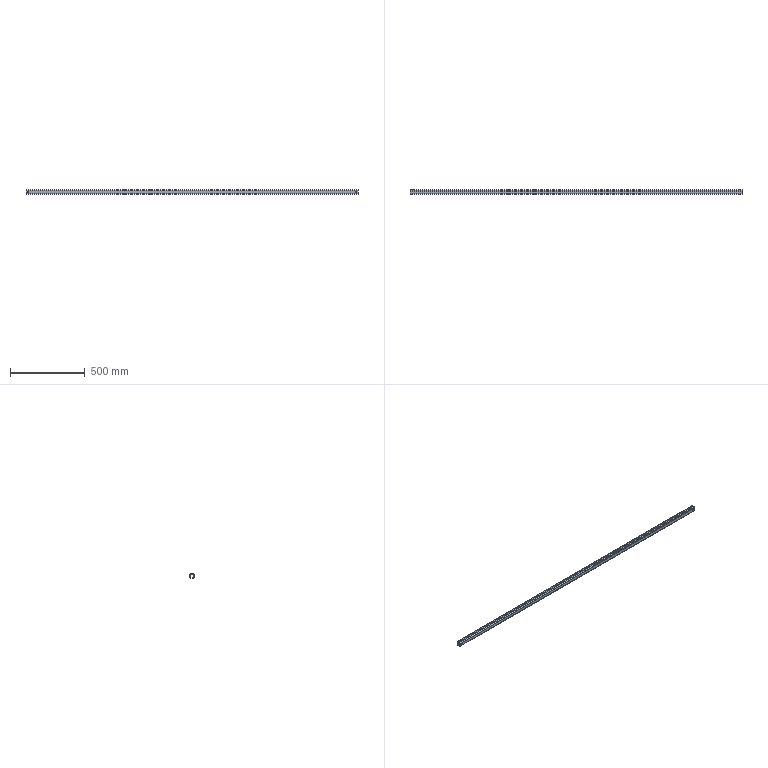Part | NX | features solid 2 | 1 solid | 30 faces | box 2220 x 30 x 30 mm | volume 666162 mm3 | cylinder 16 | plane 14 | commonest cylinder face diameters 6 x4 10 x4 12 x4 15 x4
STEP:
#1=CARTESIAN_POINT('',(1095.,-620.,42.5));
#2=VERTEX_POINT('',#1);
#3=CARTESIAN_POINT('',(1095.,-623.,42.5));
#4=VERTEX_POINT('',#3);
#5=CARTESIAN_POINT('',(1095.,-620.,42.5));
#6=DIRECTION('',(0.,-1.,0.));
#7=VECTOR('',#6,1000.);
#8=LINE('',#5,#7);
#9=EDGE_CURVE('',#2,#4,#8,.T.);
#10=ORIENTED_EDGE('',*,*,#9,.F.);
#11=CARTESIAN_POINT('',(1095.,-620.,57.5));
#12=VERTEX_POINT('',#11);
#13=CARTESIAN_POINT('',(1095.,-620.,50.));
#14=DIRECTION('',(0.,-1.,0.));
#15=DIRECTION('',(0.,0.,1.));
#16=AXIS2_PLACEMENT_3D('',#13,#14,#15);
#17=CIRCLE('',#16,7.5);
#18=EDGE_CURVE('',#12,#2,#17,.T.);
#19=ORIENTED_EDGE('',*,*,#18,.F.);
#20=CARTESIAN_POINT('',(1095.,-623.,57.5));
#21=VERTEX_POINT('',#20);
#22=CARTESIAN_POINT('',(1095.,-620.,57.5));
#23=DIRECTION('',(0.,-1.,0.));
#24=VECTOR('',#23,1000.);
#25=LINE('',#22,#24);
#26=EDGE_CURVE('',#21,#12,#25,.F.);
#27=ORIENTED_EDGE('',*,*,#26,.F.);
#28=CARTESIAN_POINT('',(1095.,-623.,50.));
#29=DIRECTION('',(0.,1.,0.));
#30=DIRECTION('',(0.,0.,1.));
#31=AXIS2_PLACEMENT_3D('',#28,#29,#30);
#32=CIRCLE('',#31,7.5);
#33=EDGE_CURVE('',#4,#21,#32,.T.);
#34=ORIENTED_EDGE('',*,*,#33,.F.);
#35=EDGE_LOOP('',(#10,#19,#27,#34));
#36=FACE_BOUND('',#35,.T.);
#37=CARTESIAN_POINT('',(1095.,-620.,50.));
#38=DIRECTION('',(0.,-1.,0.));
#39=DIRECTION('',(0.,0.,1.));
#40=AXIS2_PLACEMENT_3D('',#37,#38,#39);
#41=CYLINDRICAL_SURFACE('',#40,7.5);
#42=ADVANCED_FACE('',(#36),#41,.F.);
#43=CARTESIAN_POINT('',(1095.,-650.,45.));
#44=VERTEX_POINT('',#43);
#45=CARTESIAN_POINT('',(1095.,-647.,45.));
#46=VERTEX_POINT('',#45);
#47=CARTESIAN_POINT('',(1095.,-2849.405,45.));
#48=DIRECTION('',(0.,1.,0.));
#49=VECTOR('',#48,1000.);
#50=LINE('',#47,#49);
#51=EDGE_CURVE('',#44,#46,#50,.T.);
#52=ORIENTED_EDGE('',*,*,#51,.F.);
#53=CARTESIAN_POINT('',(1095.,-650.,55.));
#54=VERTEX_POINT('',#53);
#55=CARTESIAN_POINT('',(1095.,-650.,50.));
#56=DIRECTION('',(0.,-1.,0.));
#57=DIRECTION('',(0.,0.,-1.));
#58=AXIS2_PLACEMENT_3D('',#55,#56,#57);
#59=CIRCLE('',#58,5.);
#60=EDGE_CURVE('',#44,#54,#59,.T.);
#61=ORIENTED_EDGE('',*,*,#60,.T.);
#62=CARTESIAN_POINT('',(1095.,-647.,55.));
#63=VERTEX_POINT('',#62);
#64=CARTESIAN_POINT('',(1095.,-2849.405,55.));
#65=DIRECTION('',(0.,1.,0.));
#66=VECTOR('',#65,1000.);
#67=LINE('',#64,#66);
#68=EDGE_CURVE('',#63,#54,#67,.F.);
#69=ORIENTED_EDGE('',*,*,#68,.F.);
#70=CARTESIAN_POINT('',(1095.,-647.,50.));
#71=DIRECTION('',(0.,-1.,0.));
#72=DIRECTION('',(0.,0.,-1.));
#73=AXIS2_PLACEMENT_3D('',#70,#71,#72);
#74=CIRCLE('',#73,5.);
#75=EDGE_CURVE('',#46,#63,#74,.T.);
#76=ORIENTED_EDGE('',*,*,#75,.F.);
#77=EDGE_LOOP('',(#52,#61,#69,#76));
#78=FACE_BOUND('',#77,.T.);
#79=CARTESIAN_POINT('',(1095.,-2849.405,50.));
#80=DIRECTION('',(0.,1.,0.));
#81=DIRECTION('',(0.,0.,1.));
#82=AXIS2_PLACEMENT_3D('',#79,#80,#81);
#83=CYLINDRICAL_SURFACE('',#82,5.);
#84=ADVANCED_FACE('',(#78),#83,.F.);
#85=CARTESIAN_POINT('',(-1095.,-620.,42.5));
#86=VERTEX_POINT('',#85);
#87=CARTESIAN_POINT('',(-1095.,-623.,42.5));
#88=VERTEX_POINT('',#87);
#89=CARTESIAN_POINT('',(-1095.,-620.,42.5));
#90=DIRECTION('',(0.,-1.,0.));
#91=VECTOR('',#90,1000.);
#92=LINE('',#89,#91);
#93=EDGE_CURVE('',#86,#88,#92,.T.);
#94=ORIENTED_EDGE('',*,*,#93,.F.);
#95=CARTESIAN_POINT('',(-1095.,-620.,57.5));
#96=VERTEX_POINT('',#95);
#97=CARTESIAN_POINT('',(-1095.,-620.,50.));
#98=DIRECTION('',(0.,-1.,0.));
#99=DIRECTION('',(0.,0.,1.));
#100=AXIS2_PLACEMENT_3D('',#97,#98,#99);
#101=CIRCLE('',#100,7.5);
#102=EDGE_CURVE('',#96,#86,#101,.T.);
#103=ORIENTED_EDGE('',*,*,#102,.F.);
#104=CARTESIAN_POINT('',(-1095.,-623.,57.5));
#105=VERTEX_POINT('',#104);
#106=CARTESIAN_POINT('',(-1095.,-620.,57.5));
#107=DIRECTION('',(0.,-1.,0.));
#108=VECTOR('',#107,1000.);
#109=LINE('',#106,#108);
#110=EDGE_CURVE('',#105,#96,#109,.F.);
#111=ORIENTED_EDGE('',*,*,#110,.F.);
#112=CARTESIAN_POINT('',(-1095.,-623.,50.));
#113=DIRECTION('',(0.,1.,0.));
#114=DIRECTION('',(0.,0.,1.));
#115=AXIS2_PLACEMENT_3D('',#112,#113,#114);
#116=CIRCLE('',#115,7.5);
#117=EDGE_CURVE('',#88,#105,#116,.T.);
#118=ORIENTED_EDGE('',*,*,#117,.F.);
#119=EDGE_LOOP('',(#94,#103,#111,#118));
#120=FACE_BOUND('',#119,.T.);
#121=CARTESIAN_POINT('',(-1095.,-620.,50.));
#122=DIRECTION('',(0.,-1.,0.));
#123=DIRECTION('',(0.,0.,1.));
#124=AXIS2_PLACEMENT_3D('',#121,#122,#123);
#125=CYLINDRICAL_SURFACE('',#124,7.5);
#126=ADVANCED_FACE('',(#120),#125,.F.);
#127=CARTESIAN_POINT('',(-1095.,-647.,45.));
#128=VERTEX_POINT('',#127);
#129=CARTESIAN_POINT('',(-1095.,-650.,45.));
#130=VERTEX_POINT('',#129);
#131=CARTESIAN_POINT('',(-1095.,-2849.405,45.));
#132=DIRECTION('',(0.,1.,0.));
#133=VECTOR('',#132,1000.);
#134=LINE('',#131,#133);
#135=EDGE_CURVE('',#128,#130,#134,.F.);
#136=ORIENTED_EDGE('',*,*,#135,.T.);
#137=CARTESIAN_POINT('',(-1095.,-650.,55.));
#138=VERTEX_POINT('',#137);
#139=CARTESIAN_POINT('',(-1095.,-650.,50.));
#140=DIRECTION('',(0.,-1.,0.));
#141=DIRECTION('',(0.,0.,-1.));
#142=AXIS2_PLACEMENT_3D('',#139,#140,#141);
#143=CIRCLE('',#142,5.);
#144=EDGE_CURVE('',#130,#138,#143,.T.);
#145=ORIENTED_EDGE('',*,*,#144,.T.);
#146=CARTESIAN_POINT('',(-1095.,-647.,55.));
#147=VERTEX_POINT('',#146);
#148=CARTESIAN_POINT('',(-1095.,-2849.405,55.));
#149=DIRECTION('',(0.,1.,0.));
#150=VECTOR('',#149,1000.);
#151=LINE('',#148,#150);
#152=EDGE_CURVE('',#138,#147,#151,.T.);
#153=ORIENTED_EDGE('',*,*,#152,.T.);
#154=CARTESIAN_POINT('',(-1095.,-647.,50.));
#155=DIRECTION('',(0.,-1.,0.));
#156=DIRECTION('',(0.,0.,-1.));
#157=AXIS2_PLACEMENT_3D('',#154,#155,#156);
#158=CIRCLE('',#157,5.);
#159=EDGE_CURVE('',#128,#147,#158,.T.);
#160=ORIENTED_EDGE('',*,*,#159,.F.);
#161=EDGE_LOOP('',(#136,#145,#153,#160));
#162=FACE_BOUND('',#161,.T.);
#163=CARTESIAN_POINT('',(-1095.,-2849.405,50.));
#164=DIRECTION('',(0.,1.,0.));
#165=DIRECTION('',(0.,0.,1.));
#166=AXIS2_PLACEMENT_3D('',#163,#164,#165);
#167=CYLINDRICAL_SURFACE('',#166,5.);
#168=ADVANCED_FACE('',(#162),#167,.F.);
#169=CARTESIAN_POINT('',(1110.,-626.,62.));
#170=VERTEX_POINT('',#169);
#171=CARTESIAN_POINT('',(1110.,-634.99,62.));
#172=VERTEX_POINT('',#171);
#173=CARTESIAN_POINT('',(1110.,-620.,62.));
#174=DIRECTION('',(0.,-1.,0.));
#175=VECTOR('',#174,1000.);
#176=LINE('',#173,#175);
#177=EDGE_CURVE('',#170,#172,#176,.T.);
#178=ORIENTED_EDGE('',*,*,#177,.T.);
#179=CARTESIAN_POINT('',(-1110.,-634.99,62.));
#180=VERTEX_POINT('',#179);
#181=CARTESIAN_POINT('',(-1110.,-634.99,62.));
#182=DIRECTION('',(1.,0.,0.));
#183=VECTOR('',#182,1000.);
#184=LINE('',#181,#183);
#185=EDGE_CURVE('',#180,#172,#184,.T.);
#186=ORIENTED_EDGE('',*,*,#185,.F.);
#187=CARTESIAN_POINT('',(-1110.,-626.,62.));
#188=VERTEX_POINT('',#187);
#189=CARTESIAN_POINT('',(-1110.,-620.,62.));
#190=DIRECTION('',(0.,-1.,0.));
#191=VECTOR('',#190,1000.);
#192=LINE('',#189,#191);
#193=EDGE_CURVE('',#188,#180,#192,.T.);
#194=ORIENTED_EDGE('',*,*,#193,.F.);
#195=CARTESIAN_POINT('',(-1110.,-626.,62.));
#196=DIRECTION('',(1.,0.,0.));
#197=VECTOR('',#196,1000.);
#198=LINE('',#195,#197);
#199=EDGE_CURVE('',#188,#170,#198,.T.);
#200=ORIENTED_EDGE('',*,*,#199,.T.);
#201=EDGE_LOOP('',(#178,#186,#194,#200));
#202=FACE_BOUND('',#201,.T.);
#203=CARTESIAN_POINT('',(-1110.,-620.,62.));
#204=DIRECTION('',(0.,0.,1.));
#205=DIRECTION('',(0.,-1.,0.));
#206=AXIS2_PLACEMENT_3D('',#203,#204,#205);
#207=PLANE('',#206);
#208=ADVANCED_FACE('',(#202),#207,.F.);
#209=CARTESIAN_POINT('',(1110.,-623.,59.));
#210=VERTEX_POINT('',#209);
#211=CARTESIAN_POINT('',(1110.,-626.,59.));
#212=DIRECTION('',(1.,0.,0.));
#213=DIRECTION('',(0.,0.,-1.));
#214=AXIS2_PLACEMENT_3D('',#211,#212,#213);
#215=CIRCLE('',#214,3.);
#216=EDGE_CURVE('',#210,#170,#215,.T.);
#217=ORIENTED_EDGE('',*,*,#216,.T.);
#218=ORIENTED_EDGE('',*,*,#199,.F.);
#219=CARTESIAN_POINT('',(-1110.,-623.,59.));
#220=VERTEX_POINT('',#219);
#221=CARTESIAN_POINT('',(-1110.,-626.,59.));
#222=DIRECTION('',(1.,0.,0.));
#223=DIRECTION('',(0.,0.,-1.));
#224=AXIS2_PLACEMENT_3D('',#221,#222,#223);
#225=CIRCLE('',#224,3.);
#226=EDGE_CURVE('',#220,#188,#225,.T.);
#227=ORIENTED_EDGE('',*,*,#226,.F.);
#228=CARTESIAN_POINT('',(-1110.,-623.,59.));
#229=DIRECTION('',(1.,0.,0.));
#230=VECTOR('',#229,1000.);
#231=LINE('',#228,#230);
#232=EDGE_CURVE('',#220,#210,#231,.T.);
#233=ORIENTED_EDGE('',*,*,#232,.T.);
#234=EDGE_LOOP('',(#217,#218,#227,#233));
#235=FACE_BOUND('',#234,.T.);
#236=CARTESIAN_POINT('',(-1110.,-626.,59.));
#237=DIRECTION('',(1.,0.,0.));
#238=DIRECTION('',(0.,0.,-1.));
#239=AXIS2_PLACEMENT_3D('',#236,#237,#238);
#240=CYLINDRICAL_SURFACE('',#239,3.);
#241=ADVANCED_FACE('',(#235),#240,.F.);
#242=CARTESIAN_POINT('',(-1095.,-623.,50.));
#243=DIRECTION('',(0.,1.,0.));
#244=DIRECTION('',(0.,0.,1.));
#245=AXIS2_PLACEMENT_3D('',#242,#243,#244);
#246=CIRCLE('',#245,7.5);
#247=EDGE_CURVE('',#105,#88,#246,.T.);
#248=ORIENTED_EDGE('',*,*,#247,.T.);
#249=ORIENTED_EDGE('',*,*,#117,.T.);
#250=EDGE_LOOP('',(#248,#249));
#251=FACE_BOUND('',#250,.T.);
#252=CARTESIAN_POINT('',(1095.,-623.,50.));
#253=DIRECTION('',(0.,1.,0.));
#254=DIRECTION('',(0.,0.,1.));
#255=AXIS2_PLACEMENT_3D('',#252,#253,#254);
#256=CIRCLE('',#255,7.5);
#257=EDGE_CURVE('',#21,#4,#256,.T.);
#258=ORIENTED_EDGE('',*,*,#257,.T.);
#259=ORIENTED_EDGE('',*,*,#33,.T.);
#260=EDGE_LOOP('',(#258,#259));
#261=FACE_BOUND('',#260,.T.);
#262=CARTESIAN_POINT('',(1110.,-623.,41.));
#263=VERTEX_POINT('',#262);
#264=CARTESIAN_POINT('',(1110.,-623.,35.));
#265=DIRECTION('',(0.,0.,1.));
#266=VECTOR('',#265,1000.);
#267=LINE('',#264,#266);
#268=EDGE_CURVE('',#263,#210,#267,.T.);
#269=ORIENTED_EDGE('',*,*,#268,.T.);
#270=ORIENTED_EDGE('',*,*,#232,.F.);
#271=CARTESIAN_POINT('',(-1110.,-623.,41.));
#272=VERTEX_POINT('',#271);
#273=CARTESIAN_POINT('',(-1110.,-623.,35.));
#274=DIRECTION('',(0.,0.,1.));
#275=VECTOR('',#274,1000.);
#276=LINE('',#273,#275);
#277=EDGE_CURVE('',#272,#220,#276,.T.);
#278=ORIENTED_EDGE('',*,*,#277,.F.);
#279=CARTESIAN_POINT('',(-1110.,-623.,41.));
#280=DIRECTION('',(1.,0.,0.));
#281=VECTOR('',#280,1000.);
#282=LINE('',#279,#281);
#283=EDGE_CURVE('',#272,#263,#282,.T.);
#284=ORIENTED_EDGE('',*,*,#283,.T.);
#285=EDGE_LOOP('',(#269,#270,#278,#284));
#286=FACE_BOUND('',#285,.T.);
#287=CARTESIAN_POINT('',(-1110.,-623.,35.));
#288=DIRECTION('',(0.,1.,0.));
#289=DIRECTION('',(0.,0.,-1.));
#290=AXIS2_PLACEMENT_3D('',#287,#288,#289);
#291=PLANE('',#290);
#292=ADVANCED_FACE('',(#251,#261,#286),#291,.F.);
#293=CARTESIAN_POINT('',(1110.,-626.,38.));
#294=VERTEX_POINT('',#293);
#295=CARTESIAN_POINT('',(1110.,-626.,41.));
#296=DIRECTION('',(1.,0.,0.));
#297=DIRECTION('',(0.,0.,-1.));
#298=AXIS2_PLACEMENT_3D('',#295,#296,#297);
#299=CIRCLE('',#298,3.);
#300=EDGE_CURVE('',#294,#263,#299,.T.);
#301=ORIENTED_EDGE('',*,*,#300,.T.);
#302=ORIENTED_EDGE('',*,*,#283,.F.);
#303=CARTESIAN_POINT('',(-1110.,-626.,38.));
#304=VERTEX_POINT('',#303);
#305=CARTESIAN_POINT('',(-1110.,-626.,41.));
#306=DIRECTION('',(1.,0.,0.));
#307=DIRECTION('',(0.,0.,-1.));
#308=AXIS2_PLACEMENT_3D('',#305,#306,#307);
#309=CIRCLE('',#308,3.);
#310=EDGE_CURVE('',#304,#272,#309,.T.);
#311=ORIENTED_EDGE('',*,*,#310,.F.);
#312=CARTESIAN_POINT('',(-1110.,-626.,38.));
#313=DIRECTION('',(1.,0.,0.));
#314=VECTOR('',#313,1000.);
#315=LINE('',#312,#314);
#316=EDGE_CURVE('',#304,#294,#315,.T.);
#317=ORIENTED_EDGE('',*,*,#316,.T.);
#318=EDGE_LOOP('',(#301,#302,#311,#317));
#319=FACE_BOUND('',#318,.T.);
#320=CARTESIAN_POINT('',(-1110.,-626.,41.));
#321=DIRECTION('',(1.,0.,0.));
#322=DIRECTION('',(0.,0.,-1.));
#323=AXIS2_PLACEMENT_3D('',#320,#321,#322);
#324=CYLINDRICAL_SURFACE('',#323,3.);
#325=ADVANCED_FACE('',(#319),#324,.F.);
#326=CARTESIAN_POINT('',(1110.,-644.,38.));
#327=VERTEX_POINT('',#326);
#328=CARTESIAN_POINT('',(1110.,-650.,38.));
#329=DIRECTION('',(0.,1.,0.));
#330=VECTOR('',#329,1000.);
#331=LINE('',#328,#330);
#332=EDGE_CURVE('',#327,#294,#331,.T.);
#333=ORIENTED_EDGE('',*,*,#332,.T.);
#334=ORIENTED_EDGE('',*,*,#316,.F.);
#335=CARTESIAN_POINT('',(-1110.,-644.,38.));
#336=VERTEX_POINT('',#335);
#337=CARTESIAN_POINT('',(-1110.,-650.,38.));
#338=DIRECTION('',(0.,1.,0.));
#339=VECTOR('',#338,1000.);
#340=LINE('',#337,#339);
#341=EDGE_CURVE('',#336,#304,#340,.T.);
#342=ORIENTED_EDGE('',*,*,#341,.F.);
#343=CARTESIAN_POINT('',(-1110.,-644.,38.));
#344=DIRECTION('',(1.,0.,0.));
#345=VECTOR('',#344,1000.);
#346=LINE('',#343,#345);
#347=EDGE_CURVE('',#336,#327,#346,.T.);
#348=ORIENTED_EDGE('',*,*,#347,.T.);
#349=EDGE_LOOP('',(#333,#334,#342,#348));
#350=FACE_BOUND('',#349,.T.);
#351=CARTESIAN_POINT('',(-1110.,-650.,38.));
#352=DIRECTION('',(0.,0.,-1.));
#353=DIRECTION('',(0.,-1.,0.));
#354=AXIS2_PLACEMENT_3D('',#351,#352,#353);
#355=PLANE('',#354);
#356=ADVANCED_FACE('',(#350),#355,.F.);
#357=CARTESIAN_POINT('',(1110.,-647.,41.));
#358=VERTEX_POINT('',#357);
#359=CARTESIAN_POINT('',(1110.,-644.,41.));
#360=DIRECTION('',(1.,0.,0.));
#361=DIRECTION('',(0.,0.,-1.));
#362=AXIS2_PLACEMENT_3D('',#359,#360,#361);
#363=CIRCLE('',#362,3.);
#364=EDGE_CURVE('',#358,#327,#363,.T.);
#365=ORIENTED_EDGE('',*,*,#364,.T.);
#366=ORIENTED_EDGE('',*,*,#347,.F.);
#367=CARTESIAN_POINT('',(-1110.,-647.,41.));
#368=VERTEX_POINT('',#367);
#369=CARTESIAN_POINT('',(-1110.,-644.,41.));
#370=DIRECTION('',(1.,0.,0.));
#371=DIRECTION('',(0.,0.,-1.));
#372=AXIS2_PLACEMENT_3D('',#369,#370,#371);
#373=CIRCLE('',#372,3.);
#374=EDGE_CURVE('',#368,#336,#373,.T.);
#375=ORIENTED_EDGE('',*,*,#374,.F.);
#376=CARTESIAN_POINT('',(-1110.,-647.,41.));
#377=DIRECTION('',(1.,0.,0.));
#378=VECTOR('',#377,1000.);
#379=LINE('',#376,#378);
#380=EDGE_CURVE('',#368,#358,#379,.T.);
#381=ORIENTED_EDGE('',*,*,#380,.T.);
#382=EDGE_LOOP('',(#365,#366,#375,#381));
#383=FACE_BOUND('',#382,.T.);
#384=CARTESIAN_POINT('',(-1110.,-644.,41.));
#385=DIRECTION('',(1.,0.,0.));
#386=DIRECTION('',(0.,0.,-1.));
#387=AXIS2_PLACEMENT_3D('',#384,#385,#386);
#388=CYLINDRICAL_SURFACE('',#387,3.);
#389=ADVANCED_FACE('',(#383),#388,.F.);
#390=CARTESIAN_POINT('',(-1095.,-647.,50.));
#391=DIRECTION('',(0.,-1.,0.));
#392=DIRECTION('',(0.,0.,-1.));
#393=AXIS2_PLACEMENT_3D('',#390,#391,#392);
#394=CIRCLE('',#393,5.);
#395=EDGE_CURVE('',#147,#128,#394,.T.);
#396=ORIENTED_EDGE('',*,*,#395,.T.);
#397=ORIENTED_EDGE('',*,*,#159,.T.);
#398=EDGE_LOOP('',(#396,#397));
#399=FACE_BOUND('',#398,.T.);
#400=CARTESIAN_POINT('',(1095.,-647.,50.));
#401=DIRECTION('',(0.,-1.,0.));
#402=DIRECTION('',(0.,0.,-1.));
#403=AXIS2_PLACEMENT_3D('',#400,#401,#402);
#404=CIRCLE('',#403,5.);
#405=EDGE_CURVE('',#63,#46,#404,.T.);
#406=ORIENTED_EDGE('',*,*,#405,.T.);
#407=ORIENTED_EDGE('',*,*,#75,.T.);
#408=EDGE_LOOP('',(#406,#407));
#409=FACE_BOUND('',#408,.T.);
#410=CARTESIAN_POINT('',(1110.,-647.,59.));
#411=VERTEX_POINT('',#410);
#412=CARTESIAN_POINT('',(1110.,-647.,65.));
#413=DIRECTION('',(0.,0.,-1.));
#414=VECTOR('',#413,1000.);
#415=LINE('',#412,#414);
#416=EDGE_CURVE('',#411,#358,#415,.T.);
#417=ORIENTED_EDGE('',*,*,#416,.T.);
#418=ORIENTED_EDGE('',*,*,#380,.F.);
#419=CARTESIAN_POINT('',(-1110.,-647.,59.));
#420=VERTEX_POINT('',#419);
#421=CARTESIAN_POINT('',(-1110.,-647.,65.));
#422=DIRECTION('',(0.,0.,-1.));
#423=VECTOR('',#422,1000.);
#424=LINE('',#421,#423);
#425=EDGE_CURVE('',#420,#368,#424,.T.);
#426=ORIENTED_EDGE('',*,*,#425,.F.);
#427=CARTESIAN_POINT('',(-1110.,-647.,59.));
#428=DIRECTION('',(1.,0.,0.));
#429=VECTOR('',#428,1000.);
#430=LINE('',#427,#429);
#431=EDGE_CURVE('',#420,#411,#430,.T.);
#432=ORIENTED_EDGE('',*,*,#431,.T.);
#433=EDGE_LOOP('',(#417,#418,#426,#432));
#434=FACE_BOUND('',#433,.T.);
#435=CARTESIAN_POINT('',(-1110.,-647.,65.));
#436=DIRECTION('',(0.,-1.,0.));
#437=DIRECTION('',(0.,0.,-1.));
#438=AXIS2_PLACEMENT_3D('',#435,#436,#437);
#439=PLANE('',#438);
#440=ADVANCED_FACE('',(#399,#409,#434),#439,.F.);
#441=CARTESIAN_POINT('',(1110.,-644.,62.));
#442=VERTEX_POINT('',#441);
#443=CARTESIAN_POINT('',(1110.,-644.,59.));
#444=DIRECTION('',(1.,0.,0.));
#445=DIRECTION('',(0.,0.,-1.));
#446=AXIS2_PLACEMENT_3D('',#443,#444,#445);
#447=CIRCLE('',#446,3.);
#448=EDGE_CURVE('',#442,#411,#447,.T.);
#449=ORIENTED_EDGE('',*,*,#448,.T.);
#450=ORIENTED_EDGE('',*,*,#431,.F.);
#451=CARTESIAN_POINT('',(-1110.,-644.,62.));
#452=VERTEX_POINT('',#451);
#453=CARTESIAN_POINT('',(-1110.,-644.,59.));
#454=DIRECTION('',(1.,0.,0.));
#455=DIRECTION('',(0.,0.,-1.));
#456=AXIS2_PLACEMENT_3D('',#453,#454,#455);
#457=CIRCLE('',#456,3.);
#458=EDGE_CURVE('',#452,#420,#457,.T.);
#459=ORIENTED_EDGE('',*,*,#458,.F.);
#460=CARTESIAN_POINT('',(-1110.,-644.,62.));
#461=DIRECTION('',(1.,0.,0.));
#462=VECTOR('',#461,1000.);
#463=LINE('',#460,#462);
#464=EDGE_CURVE('',#452,#442,#463,.T.);
#465=ORIENTED_EDGE('',*,*,#464,.T.);
#466=EDGE_LOOP('',(#449,#450,#459,#465));
#467=FACE_BOUND('',#466,.T.);
#468=CARTESIAN_POINT('',(-1110.,-644.,59.));
#469=DIRECTION('',(1.,0.,0.));
#470=DIRECTION('',(0.,0.,-1.));
#471=AXIS2_PLACEMENT_3D('',#468,#469,#470);
#472=CYLINDRICAL_SURFACE('',#471,3.);
#473=ADVANCED_FACE('',(#467),#472,.F.);
#474=CARTESIAN_POINT('',(1110.,-635.01,62.));
#475=VERTEX_POINT('',#474);
#476=CARTESIAN_POINT('',(1110.,-635.01,62.));
#477=DIRECTION('',(0.,-1.,0.));
#478=VECTOR('',#477,1000.);
#479=LINE('',#476,#478);
#480=EDGE_CURVE('',#475,#442,#479,.T.);
#481=ORIENTED_EDGE('',*,*,#480,.T.);
#482=ORIENTED_EDGE('',*,*,#464,.F.);
#483=CARTESIAN_POINT('',(-1110.,-635.01,62.));
#484=VERTEX_POINT('',#483);
#485=CARTESIAN_POINT('',(-1110.,-635.01,62.));
#486=DIRECTION('',(0.,-1.,0.));
#487=VECTOR('',#486,1000.);
#488=LINE('',#485,#487);
#489=EDGE_CURVE('',#484,#452,#488,.T.);
#490=ORIENTED_EDGE('',*,*,#489,.F.);
#491=CARTESIAN_POINT('',(-1110.,-635.01,62.));
#492=DIRECTION('',(1.,0.,0.));
#493=VECTOR('',#492,1000.);
#494=LINE('',#491,#493);
#495=EDGE_CURVE('',#484,#475,#494,.T.);
#496=ORIENTED_EDGE('',*,*,#495,.T.);
#497=EDGE_LOOP('',(#481,#482,#490,#496));
#498=FACE_BOUND('',#497,.T.);
#499=CARTESIAN_POINT('',(-1110.,-635.01,62.));
#500=DIRECTION('',(0.,0.,1.));
#501=DIRECTION('',(0.,-1.,0.));
#502=AXIS2_PLACEMENT_3D('',#499,#500,#501);
#503=PLANE('',#502);
#504=ADVANCED_FACE('',(#498),#503,.F.);
#505=CARTESIAN_POINT('',(1110.,-626.,65.));
#506=VERTEX_POINT('',#505);
#507=CARTESIAN_POINT('',(1110.,-634.99,65.));
#508=VERTEX_POINT('',#507);
#509=CARTESIAN_POINT('',(1110.,-620.,65.));
#510=DIRECTION('',(0.,-1.,0.));
#511=VECTOR('',#510,1000.);
#512=LINE('',#509,#511);
#513=EDGE_CURVE('',#506,#508,#512,.T.);
#514=ORIENTED_EDGE('',*,*,#513,.F.);
#515=CARTESIAN_POINT('',(-1110.,-626.,65.));
#516=VERTEX_POINT('',#515);
#517=CARTESIAN_POINT('',(-1110.,-626.,65.));
#518=DIRECTION('',(1.,0.,0.));
#519=VECTOR('',#518,1000.);
#520=LINE('',#517,#519);
#521=EDGE_CURVE('',#516,#506,#520,.T.);
#522=ORIENTED_EDGE('',*,*,#521,.F.);
#523=CARTESIAN_POINT('',(-1110.,-634.99,65.));
#524=VERTEX_POINT('',#523);
#525=CARTESIAN_POINT('',(-1110.,-620.,65.));
#526=DIRECTION('',(0.,-1.,0.));
#527=VECTOR('',#526,1000.);
#528=LINE('',#525,#527);
#529=EDGE_CURVE('',#516,#524,#528,.T.);
#530=ORIENTED_EDGE('',*,*,#529,.T.);
#531=CARTESIAN_POINT('',(-1110.,-634.99,65.));
#532=DIRECTION('',(1.,0.,0.));
#533=VECTOR('',#532,1000.);
#534=LINE('',#531,#533);
#535=EDGE_CURVE('',#524,#508,#534,.T.);
#536=ORIENTED_EDGE('',*,*,#535,.T.);
#537=EDGE_LOOP('',(#514,#522,#530,#536));
#538=FACE_BOUND('',#537,.T.);
#539=CARTESIAN_POINT('',(-1110.,-620.,65.));
#540=DIRECTION('',(0.,0.,1.));
#541=DIRECTION('',(0.,-1.,0.));
#542=AXIS2_PLACEMENT_3D('',#539,#540,#541);
#543=PLANE('',#542);
#544=ADVANCED_FACE('',(#538),#543,.T.);
#545=CARTESIAN_POINT('',(1110.,-620.,59.));
#546=VERTEX_POINT('',#545);
#547=CARTESIAN_POINT('',(1110.,-626.,59.));
#548=DIRECTION('',(1.,0.,0.));
#549=DIRECTION('',(0.,-1.,0.));
#550=AXIS2_PLACEMENT_3D('',#547,#548,#549);
#551=CIRCLE('',#550,6.);
#552=EDGE_CURVE('',#546,#506,#551,.T.);
#553=ORIENTED_EDGE('',*,*,#552,.F.);
#554=CARTESIAN_POINT('',(-1110.,-620.,59.));
#555=VERTEX_POINT('',#554);
#556=CARTESIAN_POINT('',(-1110.,-620.,59.));
#557=DIRECTION('',(1.,0.,0.));
#558=VECTOR('',#557,1000.);
#559=LINE('',#556,#558);
#560=EDGE_CURVE('',#555,#546,#559,.T.);
#561=ORIENTED_EDGE('',*,*,#560,.F.);
#562=CARTESIAN_POINT('',(-1110.,-626.,59.));
#563=DIRECTION('',(1.,0.,0.));
#564=DIRECTION('',(0.,-1.,0.));
#565=AXIS2_PLACEMENT_3D('',#562,#563,#564);
#566=CIRCLE('',#565,6.);
#567=EDGE_CURVE('',#555,#516,#566,.T.);
#568=ORIENTED_EDGE('',*,*,#567,.T.);
#569=ORIENTED_EDGE('',*,*,#521,.T.);
#570=EDGE_LOOP('',(#553,#561,#568,#569));
#571=FACE_BOUND('',#570,.T.);
#572=CARTESIAN_POINT('',(-1110.,-626.,59.));
#573=DIRECTION('',(1.,0.,0.));
#574=DIRECTION('',(0.,0.,-1.));
#575=AXIS2_PLACEMENT_3D('',#572,#573,#574);
#576=CYLINDRICAL_SURFACE('',#575,6.);
#577=ADVANCED_FACE('',(#571),#576,.T.);
#578=ORIENTED_EDGE('',*,*,#102,.T.);
#579=CARTESIAN_POINT('',(-1095.,-620.,50.));
#580=DIRECTION('',(0.,-1.,0.));
#581=DIRECTION('',(0.,0.,1.));
#582=AXIS2_PLACEMENT_3D('',#579,#580,#581);
#583=CIRCLE('',#582,7.5);
#584=EDGE_CURVE('',#86,#96,#583,.T.);
#585=ORIENTED_EDGE('',*,*,#584,.T.);
#586=EDGE_LOOP('',(#578,#585));
#587=FACE_BOUND('',#586,.T.);
#588=ORIENTED_EDGE('',*,*,#18,.T.);
#589=CARTESIAN_POINT('',(1095.,-620.,50.));
#590=DIRECTION('',(0.,-1.,0.));
#591=DIRECTION('',(0.,0.,1.));
#592=AXIS2_PLACEMENT_3D('',#589,#590,#591);
#593=CIRCLE('',#592,7.5);
#594=EDGE_CURVE('',#2,#12,#593,.T.);
#595=ORIENTED_EDGE('',*,*,#594,.T.);
#596=EDGE_LOOP('',(#588,#595));
#597=FACE_BOUND('',#596,.T.);
#598=CARTESIAN_POINT('',(1110.,-620.,41.));
#599=VERTEX_POINT('',#598);
#600=CARTESIAN_POINT('',(1110.,-620.,35.));
#601=DIRECTION('',(0.,0.,1.));
#602=VECTOR('',#601,1000.);
#603=LINE('',#600,#602);
#604=EDGE_CURVE('',#599,#546,#603,.T.);
#605=ORIENTED_EDGE('',*,*,#604,.F.);
#606=CARTESIAN_POINT('',(-1110.,-620.,41.));
#607=VERTEX_POINT('',#606);
#608=CARTESIAN_POINT('',(-1110.,-620.,41.));
#609=DIRECTION('',(1.,0.,0.));
#610=VECTOR('',#609,1000.);
#611=LINE('',#608,#610);
#612=EDGE_CURVE('',#607,#599,#611,.T.);
#613=ORIENTED_EDGE('',*,*,#612,.F.);
#614=CARTESIAN_POINT('',(-1110.,-620.,35.));
#615=DIRECTION('',(0.,0.,1.));
#616=VECTOR('',#615,1000.);
#617=LINE('',#614,#616);
#618=EDGE_CURVE('',#607,#555,#617,.T.);
#619=ORIENTED_EDGE('',*,*,#618,.T.);
#620=ORIENTED_EDGE('',*,*,#560,.T.);
#621=EDGE_LOOP('',(#605,#613,#619,#620));
#622=FACE_BOUND('',#621,.T.);
#623=CARTESIAN_POINT('',(-1110.,-620.,35.));
#624=DIRECTION('',(0.,1.,0.));
#625=DIRECTION('',(0.,0.,-1.));
#626=AXIS2_PLACEMENT_3D('',#623,#624,#625);
#627=PLANE('',#626);
#628=ADVANCED_FACE('',(#587,#597,#622),#627,.T.);
#629=CARTESIAN_POINT('',(1110.,-626.,35.));
#630=VERTEX_POINT('',#629);
#631=CARTESIAN_POINT('',(1110.,-626.,41.));
#632=DIRECTION('',(1.,0.,0.));
#633=DIRECTION('',(0.,-1.,0.));
#634=AXIS2_PLACEMENT_3D('',#631,#632,#633);
#635=CIRCLE('',#634,6.);
#636=EDGE_CURVE('',#630,#599,#635,.T.);
#637=ORIENTED_EDGE('',*,*,#636,.F.);
#638=CARTESIAN_POINT('',(-1110.,-626.,35.));
#639=VERTEX_POINT('',#638);
#640=CARTESIAN_POINT('',(-1110.,-626.,35.));
#641=DIRECTION('',(1.,0.,0.));
#642=VECTOR('',#641,1000.);
#643=LINE('',#640,#642);
#644=EDGE_CURVE('',#639,#630,#643,.T.);
#645=ORIENTED_EDGE('',*,*,#644,.F.);
#646=CARTESIAN_POINT('',(-1110.,-626.,41.));
#647=DIRECTION('',(1.,0.,0.));
#648=DIRECTION('',(0.,-1.,0.));
#649=AXIS2_PLACEMENT_3D('',#646,#647,#648);
#650=CIRCLE('',#649,6.);
#651=EDGE_CURVE('',#639,#607,#650,.T.);
#652=ORIENTED_EDGE('',*,*,#651,.T.);
#653=ORIENTED_EDGE('',*,*,#612,.T.);
#654=EDGE_LOOP('',(#637,#645,#652,#653));
#655=FACE_BOUND('',#654,.T.);
#656=CARTESIAN_POINT('',(-1110.,-626.,41.));
#657=DIRECTION('',(1.,0.,0.));
#658=DIRECTION('',(0.,0.,-1.));
#659=AXIS2_PLACEMENT_3D('',#656,#657,#658);
#660=CYLINDRICAL_SURFACE('',#659,6.);
#661=ADVANCED_FACE('',(#655),#660,.T.);
#662=CARTESIAN_POINT('',(1110.,-644.,35.));
#663=VERTEX_POINT('',#662);
#664=CARTESIAN_POINT('',(1110.,-650.,35.));
#665=DIRECTION('',(0.,1.,0.));
#666=VECTOR('',#665,1000.);
#667=LINE('',#664,#666);
#668=EDGE_CURVE('',#663,#630,#667,.T.);
#669=ORIENTED_EDGE('',*,*,#668,.F.);
#670=CARTESIAN_POINT('',(-1110.,-644.,35.));
#671=VERTEX_POINT('',#670);
#672=CARTESIAN_POINT('',(-1110.,-644.,35.));
#673=DIRECTION('',(1.,0.,0.));
#674=VECTOR('',#673,1000.);
#675=LINE('',#672,#674);
#676=EDGE_CURVE('',#671,#663,#675,.T.);
#677=ORIENTED_EDGE('',*,*,#676,.F.);
#678=CARTESIAN_POINT('',(-1110.,-650.,35.));
#679=DIRECTION('',(0.,1.,0.));
#680=VECTOR('',#679,1000.);
#681=LINE('',#678,#680);
#682=EDGE_CURVE('',#671,#639,#681,.T.);
#683=ORIENTED_EDGE('',*,*,#682,.T.);
#684=ORIENTED_EDGE('',*,*,#644,.T.);
#685=EDGE_LOOP('',(#669,#677,#683,#684));
#686=FACE_BOUND('',#685,.T.);
#687=CARTESIAN_POINT('',(-1110.,-650.,35.));
#688=DIRECTION('',(0.,0.,-1.));
#689=DIRECTION('',(0.,-1.,0.));
#690=AXIS2_PLACEMENT_3D('',#687,#688,#689);
#691=PLANE('',#690);
#692=ADVANCED_FACE('',(#686),#691,.T.);
#693=CARTESIAN_POINT('',(1110.,-650.,41.));
#694=VERTEX_POINT('',#693);
#695=CARTESIAN_POINT('',(1110.,-644.,41.));
#696=DIRECTION('',(1.,0.,0.));
#697=DIRECTION('',(0.,-1.,0.));
#698=AXIS2_PLACEMENT_3D('',#695,#696,#697);
#699=CIRCLE('',#698,6.);
#700=EDGE_CURVE('',#694,#663,#699,.T.);
#701=ORIENTED_EDGE('',*,*,#700,.F.);
#702=CARTESIAN_POINT('',(-1110.,-650.,41.));
#703=VERTEX_POINT('',#702);
#704=CARTESIAN_POINT('',(-1110.,-650.,41.));
#705=DIRECTION('',(1.,0.,0.));
#706=VECTOR('',#705,1000.);
#707=LINE('',#704,#706);
#708=EDGE_CURVE('',#703,#694,#707,.T.);
#709=ORIENTED_EDGE('',*,*,#708,.F.);
#710=CARTESIAN_POINT('',(-1110.,-644.,41.));
#711=DIRECTION('',(1.,0.,0.));
#712=DIRECTION('',(0.,-1.,0.));
#713=AXIS2_PLACEMENT_3D('',#710,#711,#712);
#714=CIRCLE('',#713,6.);
#715=EDGE_CURVE('',#703,#671,#714,.T.);
#716=ORIENTED_EDGE('',*,*,#715,.T.);
#717=ORIENTED_EDGE('',*,*,#676,.T.);
#718=EDGE_LOOP('',(#701,#709,#716,#717));
#719=FACE_BOUND('',#718,.T.);
#720=CARTESIAN_POINT('',(-1110.,-644.,41.));
#721=DIRECTION('',(1.,0.,0.));
#722=DIRECTION('',(0.,0.,-1.));
#723=AXIS2_PLACEMENT_3D('',#720,#721,#722);
#724=CYLINDRICAL_SURFACE('',#723,6.);
#725=ADVANCED_FACE('',(#719),#724,.T.);
#726=CARTESIAN_POINT('',(-1095.,-650.,50.));
#727=DIRECTION('',(0.,-1.,0.));
#728=DIRECTION('',(0.,0.,-1.));
#729=AXIS2_PLACEMENT_3D('',#726,#727,#728);
#730=CIRCLE('',#729,5.);
#731=EDGE_CURVE('',#138,#130,#730,.T.);
#732=ORIENTED_EDGE('',*,*,#731,.F.);
#733=ORIENTED_EDGE('',*,*,#144,.F.);
#734=EDGE_LOOP('',(#732,#733));
#735=FACE_BOUND('',#734,.T.);
#736=CARTESIAN_POINT('',(1095.,-650.,50.));
#737=DIRECTION('',(0.,-1.,0.));
#738=DIRECTION('',(0.,0.,-1.));
#739=AXIS2_PLACEMENT_3D('',#736,#737,#738);
#740=CIRCLE('',#739,5.);
#741=EDGE_CURVE('',#54,#44,#740,.T.);
#742=ORIENTED_EDGE('',*,*,#741,.F.);
#743=ORIENTED_EDGE('',*,*,#60,.F.);
#744=EDGE_LOOP('',(#742,#743));
#745=FACE_BOUND('',#744,.T.);
#746=CARTESIAN_POINT('',(1110.,-650.,59.));
#747=VERTEX_POINT('',#746);
#748=CARTESIAN_POINT('',(1110.,-650.,65.));
#749=DIRECTION('',(0.,0.,-1.));
#750=VECTOR('',#749,1000.);
#751=LINE('',#748,#750);
#752=EDGE_CURVE('',#747,#694,#751,.T.);
#753=ORIENTED_EDGE('',*,*,#752,.F.);
#754=CARTESIAN_POINT('',(-1110.,-650.,59.));
#755=VERTEX_POINT('',#754);
#756=CARTESIAN_POINT('',(-1110.,-650.,59.));
#757=DIRECTION('',(1.,0.,0.));
#758=VECTOR('',#757,1000.);
#759=LINE('',#756,#758);
#760=EDGE_CURVE('',#755,#747,#759,.T.);
#761=ORIENTED_EDGE('',*,*,#760,.F.);
#762=CARTESIAN_POINT('',(-1110.,-650.,65.));
#763=DIRECTION('',(0.,0.,-1.));
#764=VECTOR('',#763,1000.);
#765=LINE('',#762,#764);
#766=EDGE_CURVE('',#755,#703,#765,.T.);
#767=ORIENTED_EDGE('',*,*,#766,.T.);
#768=ORIENTED_EDGE('',*,*,#708,.T.);
#769=EDGE_LOOP('',(#753,#761,#767,#768));
#770=FACE_BOUND('',#769,.T.);
#771=CARTESIAN_POINT('',(-1110.,-650.,65.));
#772=DIRECTION('',(0.,-1.,0.));
#773=DIRECTION('',(0.,0.,-1.));
#774=AXIS2_PLACEMENT_3D('',#771,#772,#773);
#775=PLANE('',#774);
#776=ADVANCED_FACE('',(#735,#745,#770),#775,.T.);
#777=CARTESIAN_POINT('',(1110.,-644.,65.));
#778=VERTEX_POINT('',#777);
#779=CARTESIAN_POINT('',(1110.,-644.,59.));
#780=DIRECTION('',(1.,0.,0.));
#781=DIRECTION('',(0.,-1.,0.));
#782=AXIS2_PLACEMENT_3D('',#779,#780,#781);
#783=CIRCLE('',#782,6.);
#784=EDGE_CURVE('',#778,#747,#783,.T.);
#785=ORIENTED_EDGE('',*,*,#784,.F.);
#786=CARTESIAN_POINT('',(-1110.,-644.,65.));
#787=VERTEX_POINT('',#786);
#788=CARTESIAN_POINT('',(-1110.,-644.,65.));
#789=DIRECTION('',(1.,0.,0.));
#790=VECTOR('',#789,1000.);
#791=LINE('',#788,#790);
#792=EDGE_CURVE('',#787,#778,#791,.T.);
#793=ORIENTED_EDGE('',*,*,#792,.F.);
#794=CARTESIAN_POINT('',(-1110.,-644.,59.));
#795=DIRECTION('',(1.,0.,0.));
#796=DIRECTION('',(0.,-1.,0.));
#797=AXIS2_PLACEMENT_3D('',#794,#795,#796);
#798=CIRCLE('',#797,6.);
#799=EDGE_CURVE('',#787,#755,#798,.T.);
#800=ORIENTED_EDGE('',*,*,#799,.T.);
#801=ORIENTED_EDGE('',*,*,#760,.T.);
#802=EDGE_LOOP('',(#785,#793,#800,#801));
#803=FACE_BOUND('',#802,.T.);
#804=CARTESIAN_POINT('',(-1110.,-644.,59.));
#805=DIRECTION('',(1.,0.,0.));
#806=DIRECTION('',(0.,0.,-1.));
#807=AXIS2_PLACEMENT_3D('',#804,#805,#806);
#808=CYLINDRICAL_SURFACE('',#807,6.);
#809=ADVANCED_FACE('',(#803),#808,.T.);
#810=CARTESIAN_POINT('',(1110.,-635.01,65.));
#811=VERTEX_POINT('',#810);
#812=CARTESIAN_POINT('',(1110.,-635.01,65.));
#813=DIRECTION('',(0.,-1.,0.));
#814=VECTOR('',#813,1000.);
#815=LINE('',#812,#814);
#816=EDGE_CURVE('',#811,#778,#815,.T.);
#817=ORIENTED_EDGE('',*,*,#816,.F.);
#818=CARTESIAN_POINT('',(-1110.,-635.01,65.));
#819=VERTEX_POINT('',#818);
#820=CARTESIAN_POINT('',(-1110.,-635.01,65.));
#821=DIRECTION('',(1.,0.,0.));
#822=VECTOR('',#821,1000.);
#823=LINE('',#820,#822);
#824=EDGE_CURVE('',#819,#811,#823,.T.);
#825=ORIENTED_EDGE('',*,*,#824,.F.);
#826=CARTESIAN_POINT('',(-1110.,-635.01,65.));
#827=DIRECTION('',(0.,-1.,0.));
#828=VECTOR('',#827,1000.);
#829=LINE('',#826,#828);
#830=EDGE_CURVE('',#819,#787,#829,.T.);
#831=ORIENTED_EDGE('',*,*,#830,.T.);
#832=ORIENTED_EDGE('',*,*,#792,.T.);
#833=EDGE_LOOP('',(#817,#825,#831,#832));
#834=FACE_BOUND('',#833,.T.);
#835=CARTESIAN_POINT('',(-1110.,-635.01,65.));
#836=DIRECTION('',(0.,0.,1.));
#837=DIRECTION('',(0.,-1.,0.));
#838=AXIS2_PLACEMENT_3D('',#835,#836,#837);
#839=PLANE('',#838);
#840=ADVANCED_FACE('',(#834),#839,.T.);
#841=ORIENTED_EDGE('',*,*,#495,.F.);
#842=CARTESIAN_POINT('',(-1110.,-635.01,65.));
#843=DIRECTION('',(0.,0.,1.));
#844=VECTOR('',#843,1000.);
#845=LINE('',#842,#844);
#846=EDGE_CURVE('',#484,#819,#845,.T.);
#847=ORIENTED_EDGE('',*,*,#846,.T.);
#848=ORIENTED_EDGE('',*,*,#824,.T.);
#849=CARTESIAN_POINT('',(1110.,-635.01,65.));
#850=DIRECTION('',(0.,0.,1.));
#851=VECTOR('',#850,1000.);
#852=LINE('',#849,#851);
#853=EDGE_CURVE('',#475,#811,#852,.T.);
#854=ORIENTED_EDGE('',*,*,#853,.F.);
#855=EDGE_LOOP('',(#841,#847,#848,#854));
#856=FACE_BOUND('',#855,.T.);
#857=CARTESIAN_POINT('',(-1110.,-635.01,65.));
#858=DIRECTION('',(0.,-1.,0.));
#859=DIRECTION('',(-1.,0.,0.));
#860=AXIS2_PLACEMENT_3D('',#857,#858,#859);
#861=PLANE('',#860);
#862=ADVANCED_FACE('',(#856),#861,.F.);
#863=ORIENTED_EDGE('',*,*,#816,.T.);
#864=ORIENTED_EDGE('',*,*,#784,.T.);
#865=ORIENTED_EDGE('',*,*,#752,.T.);
#866=ORIENTED_EDGE('',*,*,#700,.T.);
#867=ORIENTED_EDGE('',*,*,#668,.T.);
#868=ORIENTED_EDGE('',*,*,#636,.T.);
#869=ORIENTED_EDGE('',*,*,#604,.T.);
#870=ORIENTED_EDGE('',*,*,#552,.T.);
#871=ORIENTED_EDGE('',*,*,#513,.T.);
#872=CARTESIAN_POINT('',(1110.,-634.99,65.));
#873=DIRECTION('',(0.,0.,1.));
#874=VECTOR('',#873,1000.);
#875=LINE('',#872,#874);
#876=EDGE_CURVE('',#172,#508,#875,.T.);
#877=ORIENTED_EDGE('',*,*,#876,.F.);
#878=ORIENTED_EDGE('',*,*,#177,.F.);
#879=ORIENTED_EDGE('',*,*,#216,.F.);
#880=ORIENTED_EDGE('',*,*,#268,.F.);
#881=ORIENTED_EDGE('',*,*,#300,.F.);
#882=ORIENTED_EDGE('',*,*,#332,.F.);
#883=ORIENTED_EDGE('',*,*,#364,.F.);
#884=ORIENTED_EDGE('',*,*,#416,.F.);
#885=ORIENTED_EDGE('',*,*,#448,.F.);
#886=ORIENTED_EDGE('',*,*,#480,.F.);
#887=ORIENTED_EDGE('',*,*,#853,.T.);
#888=EDGE_LOOP('',(#863,#864,#865,#866,#867,#868,#869,#870,#871,#877,#878,#879,#880,#881,#882,#883,#884,#885,#886,#887));
#889=FACE_BOUND('',#888,.T.);
#890=CARTESIAN_POINT('',(1110.,-635.01,65.));
#891=DIRECTION('',(-1.,0.,0.));
#892=DIRECTION('',(0.,0.,1.));
#893=AXIS2_PLACEMENT_3D('',#890,#891,#892);
#894=PLANE('',#893);
#895=ADVANCED_FACE('',(#889),#894,.F.);
#896=CARTESIAN_POINT('',(-1110.,-634.99,65.));
#897=DIRECTION('',(0.,0.,1.));
#898=VECTOR('',#897,1000.);
#899=LINE('',#896,#898);
#900=EDGE_CURVE('',#180,#524,#899,.T.);
#901=ORIENTED_EDGE('',*,*,#900,.F.);
#902=ORIENTED_EDGE('',*,*,#185,.T.);
#903=ORIENTED_EDGE('',*,*,#876,.T.);
#904=ORIENTED_EDGE('',*,*,#535,.F.);
#905=EDGE_LOOP('',(#901,#902,#903,#904));
#906=FACE_BOUND('',#905,.T.);
#907=CARTESIAN_POINT('',(-1110.,-634.99,65.));
#908=DIRECTION('',(0.,-1.,0.));
#909=DIRECTION('',(0.,0.,-1.));
#910=AXIS2_PLACEMENT_3D('',#907,#908,#909);
#911=PLANE('',#910);
#912=ADVANCED_FACE('',(#906),#911,.T.);
#913=ORIENTED_EDGE('',*,*,#529,.F.);
#914=ORIENTED_EDGE('',*,*,#567,.F.);
#915=ORIENTED_EDGE('',*,*,#618,.F.);
#916=ORIENTED_EDGE('',*,*,#651,.F.);
#917=ORIENTED_EDGE('',*,*,#682,.F.);
#918=ORIENTED_EDGE('',*,*,#715,.F.);
#919=ORIENTED_EDGE('',*,*,#766,.F.);
#920=ORIENTED_EDGE('',*,*,#799,.F.);
#921=ORIENTED_EDGE('',*,*,#830,.F.);
#922=ORIENTED_EDGE('',*,*,#846,.F.);
#923=ORIENTED_EDGE('',*,*,#489,.T.);
#924=ORIENTED_EDGE('',*,*,#458,.T.);
#925=ORIENTED_EDGE('',*,*,#425,.T.);
#926=ORIENTED_EDGE('',*,*,#374,.T.);
#927=ORIENTED_EDGE('',*,*,#341,.T.);
#928=ORIENTED_EDGE('',*,*,#310,.T.);
#929=ORIENTED_EDGE('',*,*,#277,.T.);
#930=ORIENTED_EDGE('',*,*,#226,.T.);
#931=ORIENTED_EDGE('',*,*,#193,.T.);
#932=ORIENTED_EDGE('',*,*,#900,.T.);
#933=EDGE_LOOP('',(#913,#914,#915,#916,#917,#918,#919,#920,#921,#922,#923,#924,#925,#926,#927,#928,#929,#930,#931,#932));
#934=FACE_BOUND('',#933,.T.);
#935=CARTESIAN_POINT('',(-1110.,-620.,65.));
#936=DIRECTION('',(-1.,0.,0.));
#937=DIRECTION('',(0.,0.,1.));
#938=AXIS2_PLACEMENT_3D('',#935,#936,#937);
#939=PLANE('',#938);
#940=ADVANCED_FACE('',(#934),#939,.T.);
#941=ORIENTED_EDGE('',*,*,#731,.T.);
#942=ORIENTED_EDGE('',*,*,#135,.F.);
#943=ORIENTED_EDGE('',*,*,#395,.F.);
#944=ORIENTED_EDGE('',*,*,#152,.F.);
#945=EDGE_LOOP('',(#941,#942,#943,#944));
#946=FACE_BOUND('',#945,.T.);
#947=CARTESIAN_POINT('',(-1095.,-2849.405,50.));
#948=DIRECTION('',(0.,1.,0.));
#949=DIRECTION('',(0.,0.,1.));
#950=AXIS2_PLACEMENT_3D('',#947,#948,#949);
#951=CYLINDRICAL_SURFACE('',#950,5.);
#952=ADVANCED_FACE('',(#946),#951,.F.);
#953=ORIENTED_EDGE('',*,*,#584,.F.);
#954=ORIENTED_EDGE('',*,*,#93,.T.);
#955=ORIENTED_EDGE('',*,*,#247,.F.);
#956=ORIENTED_EDGE('',*,*,#110,.T.);
#957=EDGE_LOOP('',(#953,#954,#955,#956));
#958=FACE_BOUND('',#957,.T.);
#959=CARTESIAN_POINT('',(-1095.,-620.,50.));
#960=DIRECTION('',(0.,-1.,0.));
#961=DIRECTION('',(0.,0.,1.));
#962=AXIS2_PLACEMENT_3D('',#959,#960,#961);
#963=CYLINDRICAL_SURFACE('',#962,7.5);
#964=ADVANCED_FACE('',(#958),#963,.F.);
#965=ORIENTED_EDGE('',*,*,#741,.T.);
#966=ORIENTED_EDGE('',*,*,#51,.T.);
#967=ORIENTED_EDGE('',*,*,#405,.F.);
#968=ORIENTED_EDGE('',*,*,#68,.T.);
#969=EDGE_LOOP('',(#965,#966,#967,#968));
#970=FACE_BOUND('',#969,.T.);
#971=CARTESIAN_POINT('',(1095.,-2849.405,50.));
#972=DIRECTION('',(0.,1.,0.));
#973=DIRECTION('',(0.,0.,1.));
#974=AXIS2_PLACEMENT_3D('',#971,#972,#973);
#975=CYLINDRICAL_SURFACE('',#974,5.);
#976=ADVANCED_FACE('',(#970),#975,.F.);
#977=ORIENTED_EDGE('',*,*,#594,.F.);
#978=ORIENTED_EDGE('',*,*,#9,.T.);
#979=ORIENTED_EDGE('',*,*,#257,.F.);
#980=ORIENTED_EDGE('',*,*,#26,.T.);
#981=EDGE_LOOP('',(#977,#978,#979,#980));
#982=FACE_BOUND('',#981,.T.);
#983=CARTESIAN_POINT('',(1095.,-620.,50.));
#984=DIRECTION('',(0.,-1.,0.));
#985=DIRECTION('',(0.,0.,1.));
#986=AXIS2_PLACEMENT_3D('',#983,#984,#985);
#987=CYLINDRICAL_SURFACE('',#986,7.5);
#988=ADVANCED_FACE('',(#982),#987,.F.);
#989=CLOSED_SHELL('',(#42,#84,#126,#168,#208,#241,#292,#325,#356,#389,#440,#473,#504,#544,#577,#628,#661,#692,#725,#776,#809,#840,#862,#895,#912,#940,#952,#964,#976,#988));
#990=MANIFOLD_SOLID_BREP('',#989);
#991=(LENGTH_UNIT()NAMED_UNIT(*)SI_UNIT(.MILLI.,.METRE.));
#992=UNCERTAINTY_MEASURE_WITH_UNIT(LENGTH_MEASURE(0.00001),#991,'','');
#993=(NAMED_UNIT(*)PLANE_ANGLE_UNIT()SI_UNIT($,.RADIAN.));
#994=(NAMED_UNIT(*)SI_UNIT($,.STERADIAN.)SOLID_ANGLE_UNIT());
#995=(GEOMETRIC_REPRESENTATION_CONTEXT(3)GLOBAL_UNCERTAINTY_ASSIGNED_CONTEXT((#992))GLOBAL_UNIT_ASSIGNED_CONTEXT((#991,#993,#994))REPRESENTATION_CONTEXT('',''));
#996=ADVANCED_BREP_SHAPE_REPRESENTATION('',(#990),#995);